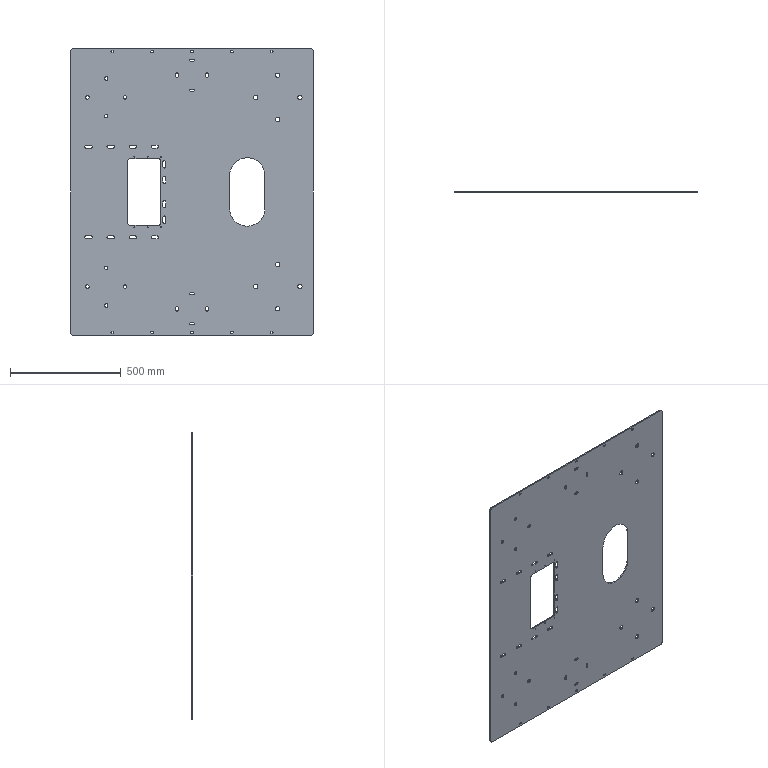Part | SolidWorks | features Cut 7, MirrorPattern 4, LPattern 3, Fillet 2, ICE 2, Extrusion 1 | 1 solid | 203 faces | box 1096 x 5 x 1296 mm | volume 6599670 mm3 | cylinder 147 | plane 56 | commonest cylinder face diameters 13.2 x28 10.5 x24 20 x24 6.6 x20 16 x16 4.4 x12